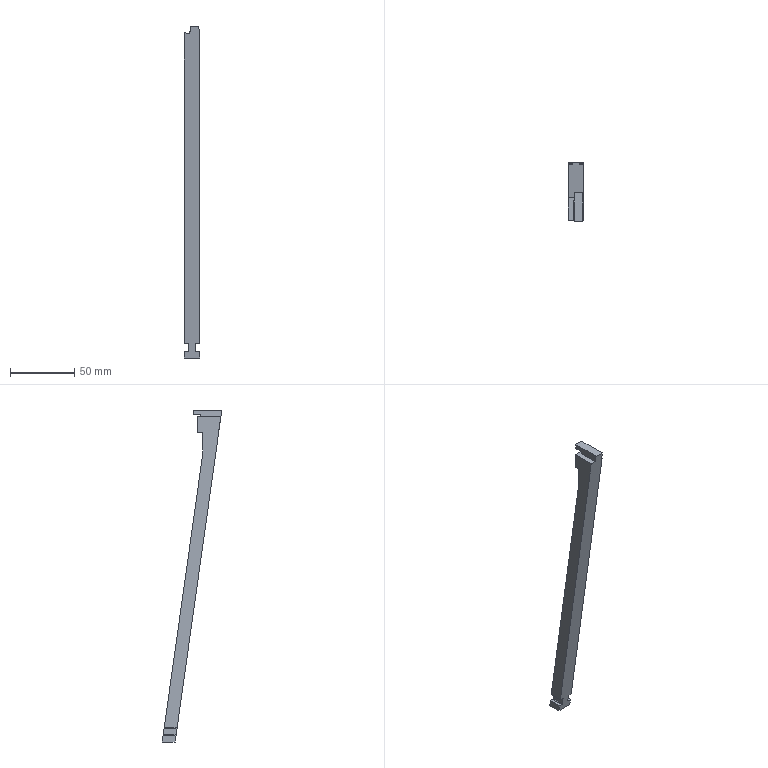Part | Creo | 1 solid | 113 faces | box 12 x 46.477 x 258.85 mm | volume 32252 mm3 | other 65 | plane 42 | cylinder 6 | commonest cylinder face diameters 1 x4 2 x1 25.401 x1